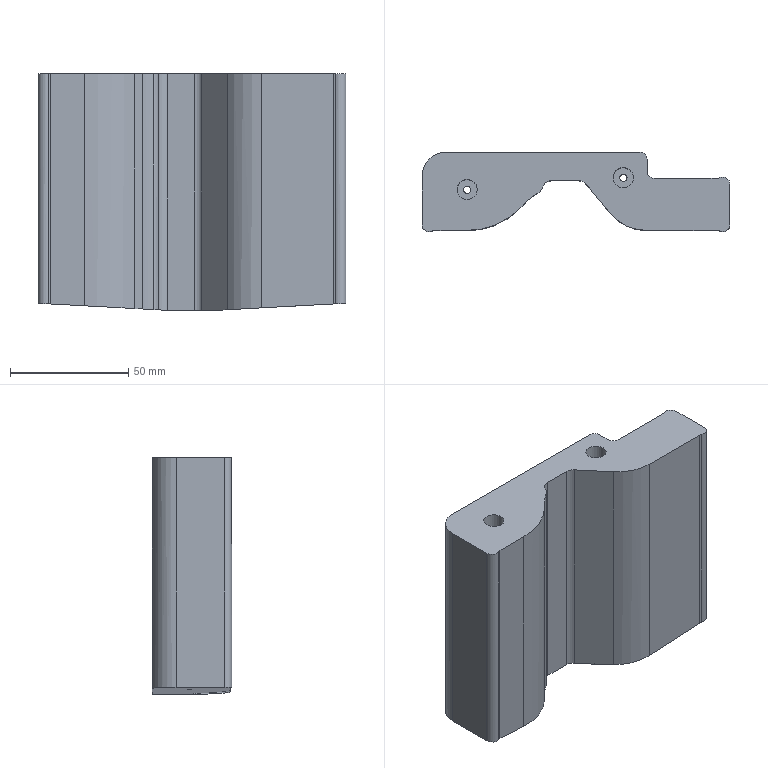Part | STEP file | lll_id242_x_t | 1 solid | 35 faces | box 130 x 33.5 x 100 mm | volume 301852 mm3 | cylinder 19 | plane 16 | commonest cylinder face diameters 6 x8 8 x3 3.1 x2 8.506 x2 20 x1 38 x1
STEP:
#1=CARTESIAN_POINT('',(669.,-7.5,-7.5));
#2=VERTEX_POINT('',#1);
#3=CARTESIAN_POINT('',(669.,-19.5,-7.5));
#4=VERTEX_POINT('',#3);
#5=CARTESIAN_POINT('',(669.,-41.,-7.5));
#6=DIRECTION('',(0.,-1.,0.));
#7=VECTOR('',#6,1.);
#8=LINE('',#5,#7);
#9=EDGE_CURVE('',#2,#4,#8,.T.);
#10=ORIENTED_EDGE('',*,*,#9,.F.);
#11=CARTESIAN_POINT('',(689.,-7.5,-7.5));
#12=VERTEX_POINT('',#11);
#13=CARTESIAN_POINT('',(781.007,-7.5,-7.5));
#14=DIRECTION('',(-1.,0.,0.));
#15=VECTOR('',#14,1.);
#16=LINE('',#13,#15);
#17=EDGE_CURVE('',#12,#2,#16,.T.);
#18=ORIENTED_EDGE('',*,*,#17,.F.);
#19=CARTESIAN_POINT('',(689.,-27.82,-7.5));
#20=VERTEX_POINT('',#19);
#21=CARTESIAN_POINT('',(689.,-41.,-7.5));
#22=DIRECTION('',(0.,1.,0.));
#23=VECTOR('',#22,1.);
#24=LINE('',#21,#23);
#25=EDGE_CURVE('',#20,#12,#24,.T.);
#26=ORIENTED_EDGE('',*,*,#25,.F.);
#27=CARTESIAN_POINT('',(683.218,-20.929,-7.5));
#28=VERTEX_POINT('',#27);
#29=CARTESIAN_POINT('',(689.435,-28.338,-7.5));
#30=DIRECTION('',(0.6428,-0.766,0.));
#31=VECTOR('',#30,1.);
#32=LINE('',#29,#31);
#33=EDGE_CURVE('',#28,#20,#32,.T.);
#34=ORIENTED_EDGE('',*,*,#33,.F.);
#35=CARTESIAN_POINT('',(680.154,-19.5,-7.5));
#36=VERTEX_POINT('',#35);
#37=CARTESIAN_POINT('',(680.154,-23.5,-7.5));
#38=DIRECTION('',(0.,0.,1.));
#39=DIRECTION('',(-1.,0.,0.));
#40=AXIS2_PLACEMENT_3D('',#37,#38,#39);
#41=CIRCLE('',#40,4.);
#42=EDGE_CURVE('',#28,#36,#41,.T.);
#43=ORIENTED_EDGE('',*,*,#42,.T.);
#44=CARTESIAN_POINT('',(781.007,-19.5,-7.5));
#45=DIRECTION('',(-1.,0.,0.));
#46=VECTOR('',#45,1.);
#47=LINE('',#44,#46);
#48=EDGE_CURVE('',#36,#4,#47,.T.);
#49=ORIENTED_EDGE('',*,*,#48,.T.);
#50=EDGE_LOOP('',(#10,#18,#26,#34,#43,#49));
#51=FACE_OUTER_BOUND('',#50,.T.);
#52=CARTESIAN_POINT('',(781.007,48.5,-7.5));
#53=DIRECTION('',(0.,0.,-1.));
#54=DIRECTION('',(1.,0.,0.));
#55=AXIS2_PLACEMENT_3D('',#52,#53,#54);
#56=PLANE('',#55);
#57=ADVANCED_FACE('',(#51),#56,.T.);
#58=CARTESIAN_POINT('',(703.253,-18.25,92.5));
#59=VERTEX_POINT('',#58);
#60=CARTESIAN_POINT('',(699.,-18.25,92.5));
#61=DIRECTION('',(0.,0.,1.));
#62=DIRECTION('',(1.,0.,0.));
#63=AXIS2_PLACEMENT_3D('',#60,#61,#62);
#64=CIRCLE('',#63,4.253);
#65=EDGE_CURVE('',#59,#59,#64,.T.);
#66=ORIENTED_EDGE('',*,*,#65,.F.);
#67=EDGE_LOOP('',(#66));
#68=FACE_BOUND('',#67,.T.);
#69=CARTESIAN_POINT('',(637.253,-23.25,92.5));
#70=VERTEX_POINT('',#69);
#71=CARTESIAN_POINT('',(633.,-23.25,92.5));
#72=DIRECTION('',(0.,0.,1.));
#73=DIRECTION('',(1.,0.,0.));
#74=AXIS2_PLACEMENT_3D('',#71,#72,#73);
#75=CIRCLE('',#74,4.253);
#76=EDGE_CURVE('',#70,#70,#75,.T.);
#77=ORIENTED_EDGE('',*,*,#76,.F.);
#78=EDGE_LOOP('',(#77));
#79=FACE_BOUND('',#78,.T.);
#80=CARTESIAN_POINT('',(708.5,-40.5,92.5));
#81=VERTEX_POINT('',#80);
#82=CARTESIAN_POINT('',(693.945,-33.713,92.5));
#83=VERTEX_POINT('',#82);
#84=CARTESIAN_POINT('',(708.5,-21.5,92.5));
#85=DIRECTION('',(0.,0.,-1.));
#86=DIRECTION('',(1.,0.,0.));
#87=AXIS2_PLACEMENT_3D('',#84,#85,#86);
#88=CIRCLE('',#87,19.);
#89=EDGE_CURVE('',#81,#83,#88,.T.);
#90=ORIENTED_EDGE('',*,*,#89,.F.);
#91=CARTESIAN_POINT('',(738.602,-40.5,92.5));
#92=VERTEX_POINT('',#91);
#93=CARTESIAN_POINT('',(741.,-40.5,92.5));
#94=DIRECTION('',(1.,0.,0.));
#95=VECTOR('',#94,1.);
#96=LINE('',#93,#95);
#97=EDGE_CURVE('',#81,#92,#96,.T.);
#98=ORIENTED_EDGE('',*,*,#97,.T.);
#99=CARTESIAN_POINT('',(739.801,-40.75,92.5));
#100=VERTEX_POINT('',#99);
#101=CARTESIAN_POINT('',(738.602,-43.5,92.5));
#102=DIRECTION('',(0.,0.,-1.));
#103=DIRECTION('',(1.,0.,0.));
#104=AXIS2_PLACEMENT_3D('',#101,#102,#103);
#105=CIRCLE('',#104,3.);
#106=EDGE_CURVE('',#92,#100,#105,.T.);
#107=ORIENTED_EDGE('',*,*,#106,.T.);
#108=CARTESIAN_POINT('',(744.,-38.,92.5));
#109=VERTEX_POINT('',#108);
#110=CARTESIAN_POINT('',(741.,-38.,92.5));
#111=DIRECTION('',(0.,0.,1.));
#112=DIRECTION('',(1.,0.,0.));
#113=AXIS2_PLACEMENT_3D('',#110,#111,#112);
#114=CIRCLE('',#113,3.);
#115=EDGE_CURVE('',#100,#109,#114,.T.);
#116=ORIENTED_EDGE('',*,*,#115,.T.);
#117=CARTESIAN_POINT('',(744.,-21.,92.5));
#118=VERTEX_POINT('',#117);
#119=CARTESIAN_POINT('',(744.,-21.,92.5));
#120=DIRECTION('',(0.,-1.,0.));
#121=VECTOR('',#120,1.);
#122=LINE('',#119,#121);
#123=EDGE_CURVE('',#118,#109,#122,.T.);
#124=ORIENTED_EDGE('',*,*,#123,.F.);
#125=CARTESIAN_POINT('',(739.801,-18.25,92.5));
#126=VERTEX_POINT('',#125);
#127=CARTESIAN_POINT('',(741.,-21.,92.5));
#128=DIRECTION('',(0.,0.,1.));
#129=DIRECTION('',(1.,0.,0.));
#130=AXIS2_PLACEMENT_3D('',#127,#128,#129);
#131=CIRCLE('',#130,3.);
#132=EDGE_CURVE('',#118,#126,#131,.T.);
#133=ORIENTED_EDGE('',*,*,#132,.T.);
#134=CARTESIAN_POINT('',(738.602,-18.5,92.5));
#135=VERTEX_POINT('',#134);
#136=CARTESIAN_POINT('',(738.602,-15.5,92.5));
#137=DIRECTION('',(0.,0.,-1.));
#138=DIRECTION('',(1.,0.,0.));
#139=AXIS2_PLACEMENT_3D('',#136,#137,#138);
#140=CIRCLE('',#139,3.);
#141=EDGE_CURVE('',#126,#135,#140,.T.);
#142=ORIENTED_EDGE('',*,*,#141,.T.);
#143=CARTESIAN_POINT('',(712.,-18.5,92.5));
#144=VERTEX_POINT('',#143);
#145=CARTESIAN_POINT('',(741.,-18.5,92.5));
#146=DIRECTION('',(1.,0.,0.));
#147=VECTOR('',#146,1.);
#148=LINE('',#145,#147);
#149=EDGE_CURVE('',#144,#135,#148,.T.);
#150=ORIENTED_EDGE('',*,*,#149,.F.);
#151=CARTESIAN_POINT('',(709.,-15.5,92.5));
#152=VERTEX_POINT('',#151);
#153=CARTESIAN_POINT('',(712.,-15.5,92.5));
#154=DIRECTION('',(0.,0.,1.));
#155=DIRECTION('',(1.,0.,0.));
#156=AXIS2_PLACEMENT_3D('',#153,#154,#155);
#157=CIRCLE('',#156,3.);
#158=EDGE_CURVE('',#152,#144,#157,.T.);
#159=ORIENTED_EDGE('',*,*,#158,.F.);
#160=CARTESIAN_POINT('',(709.,-10.5,92.5));
#161=VERTEX_POINT('',#160);
#162=CARTESIAN_POINT('',(709.,-21.,92.5));
#163=DIRECTION('',(0.,1.,0.));
#164=VECTOR('',#163,1.);
#165=LINE('',#162,#164);
#166=EDGE_CURVE('',#152,#161,#165,.T.);
#167=ORIENTED_EDGE('',*,*,#166,.T.);
#168=CARTESIAN_POINT('',(706.,-7.5,92.5));
#169=VERTEX_POINT('',#168);
#170=CARTESIAN_POINT('',(706.,-10.5,92.5));
#171=DIRECTION('',(0.,0.,1.));
#172=DIRECTION('',(1.,0.,0.));
#173=AXIS2_PLACEMENT_3D('',#170,#171,#172);
#174=CIRCLE('',#173,3.);
#175=EDGE_CURVE('',#161,#169,#174,.T.);
#176=ORIENTED_EDGE('',*,*,#175,.T.);
#177=CARTESIAN_POINT('',(624.,-7.5,92.5));
#178=VERTEX_POINT('',#177);
#179=CARTESIAN_POINT('',(741.,-7.5,92.5));
#180=DIRECTION('',(1.,0.,0.));
#181=VECTOR('',#180,1.);
#182=LINE('',#179,#181);
#183=EDGE_CURVE('',#178,#169,#182,.T.);
#184=ORIENTED_EDGE('',*,*,#183,.F.);
#185=CARTESIAN_POINT('',(614.,-17.5,92.5));
#186=VERTEX_POINT('',#185);
#187=CARTESIAN_POINT('',(624.,-17.5,92.5));
#188=DIRECTION('',(0.,0.,1.));
#189=DIRECTION('',(1.,0.,0.));
#190=AXIS2_PLACEMENT_3D('',#187,#188,#189);
#191=CIRCLE('',#190,10.);
#192=EDGE_CURVE('',#178,#186,#191,.T.);
#193=ORIENTED_EDGE('',*,*,#192,.T.);
#194=CARTESIAN_POINT('',(614.,-38.,92.5));
#195=VERTEX_POINT('',#194);
#196=CARTESIAN_POINT('',(614.,-21.,92.5));
#197=DIRECTION('',(0.,1.,0.));
#198=VECTOR('',#197,1.);
#199=LINE('',#196,#198);
#200=EDGE_CURVE('',#195,#186,#199,.T.);
#201=ORIENTED_EDGE('',*,*,#200,.F.);
#202=CARTESIAN_POINT('',(618.199,-40.75,92.5));
#203=VERTEX_POINT('',#202);
#204=CARTESIAN_POINT('',(617.,-38.,92.5));
#205=DIRECTION('',(0.,0.,-1.));
#206=DIRECTION('',(1.,0.,0.));
#207=AXIS2_PLACEMENT_3D('',#204,#205,#206);
#208=CIRCLE('',#207,3.);
#209=EDGE_CURVE('',#203,#195,#208,.T.);
#210=ORIENTED_EDGE('',*,*,#209,.F.);
#211=CARTESIAN_POINT('',(619.398,-40.5,92.5));
#212=VERTEX_POINT('',#211);
#213=CARTESIAN_POINT('',(619.398,-43.5,92.5));
#214=DIRECTION('',(0.,0.,1.));
#215=DIRECTION('',(1.,0.,0.));
#216=AXIS2_PLACEMENT_3D('',#213,#214,#215);
#217=CIRCLE('',#216,3.);
#218=EDGE_CURVE('',#212,#203,#217,.T.);
#219=ORIENTED_EDGE('',*,*,#218,.F.);
#220=CARTESIAN_POINT('',(633.574,-40.5,92.5));
#221=VERTEX_POINT('',#220);
#222=CARTESIAN_POINT('',(741.,-40.5,92.5));
#223=DIRECTION('',(1.,0.,0.));
#224=VECTOR('',#223,1.);
#225=LINE('',#222,#224);
#226=EDGE_CURVE('',#212,#221,#225,.T.);
#227=ORIENTED_EDGE('',*,*,#226,.T.);
#228=CARTESIAN_POINT('',(654.787,-31.713,92.5));
#229=VERTEX_POINT('',#228);
#230=CARTESIAN_POINT('',(633.574,-10.502,92.5));
#231=DIRECTION('',(0.,0.,-1.));
#232=DIRECTION('',(1.,0.,0.));
#233=AXIS2_PLACEMENT_3D('',#230,#231,#232);
#234=CIRCLE('',#233,29.998);
#235=EDGE_CURVE('',#229,#221,#234,.T.);
#236=ORIENTED_EDGE('',*,*,#235,.F.);
#237=CARTESIAN_POINT('',(658.142,-28.358,92.5));
#238=VERTEX_POINT('',#237);
#239=CARTESIAN_POINT('',(703.25,16.75,92.5));
#240=DIRECTION('',(0.7071,0.7071,0.));
#241=VECTOR('',#240,1.);
#242=LINE('',#239,#241);
#243=EDGE_CURVE('',#229,#238,#242,.T.);
#244=ORIENTED_EDGE('',*,*,#243,.T.);
#245=CARTESIAN_POINT('',(662.881,-24.849,92.5));
#246=VERTEX_POINT('',#245);
#247=CARTESIAN_POINT('',(672.216,-42.407,92.5));
#248=DIRECTION('',(0.,0.,-1.));
#249=DIRECTION('',(1.,0.,0.));
#250=AXIS2_PLACEMENT_3D('',#247,#248,#249);
#251=CIRCLE('',#250,19.886);
#252=EDGE_CURVE('',#238,#246,#251,.T.);
#253=ORIENTED_EDGE('',*,*,#252,.T.);
#254=CARTESIAN_POINT('',(664.848,-22.409,92.5));
#255=VERTEX_POINT('',#254);
#256=CARTESIAN_POINT('',(661.,-21.318,92.5));
#257=DIRECTION('',(0.,0.,-1.));
#258=DIRECTION('',(1.,0.,0.));
#259=AXIS2_PLACEMENT_3D('',#256,#257,#258);
#260=CIRCLE('',#259,4.);
#261=EDGE_CURVE('',#255,#246,#260,.T.);
#262=ORIENTED_EDGE('',*,*,#261,.F.);
#263=CARTESIAN_POINT('',(668.697,-19.5,92.5));
#264=VERTEX_POINT('',#263);
#265=CARTESIAN_POINT('',(668.697,-23.5,92.5));
#266=DIRECTION('',(0.,0.,1.));
#267=DIRECTION('',(1.,0.,0.));
#268=AXIS2_PLACEMENT_3D('',#265,#266,#267);
#269=CIRCLE('',#268,4.);
#270=EDGE_CURVE('',#264,#255,#269,.T.);
#271=ORIENTED_EDGE('',*,*,#270,.F.);
#272=CARTESIAN_POINT('',(680.154,-19.5,92.5));
#273=VERTEX_POINT('',#272);
#274=CARTESIAN_POINT('',(741.,-19.5,92.5));
#275=DIRECTION('',(-1.,0.,0.));
#276=VECTOR('',#275,1.);
#277=LINE('',#274,#276);
#278=EDGE_CURVE('',#273,#264,#277,.T.);
#279=ORIENTED_EDGE('',*,*,#278,.F.);
#280=CARTESIAN_POINT('',(683.218,-20.929,92.5));
#281=VERTEX_POINT('',#280);
#282=CARTESIAN_POINT('',(680.154,-23.5,92.5));
#283=DIRECTION('',(0.,0.,-1.));
#284=DIRECTION('',(1.,0.,0.));
#285=AXIS2_PLACEMENT_3D('',#282,#283,#284);
#286=CIRCLE('',#285,4.);
#287=EDGE_CURVE('',#273,#281,#286,.T.);
#288=ORIENTED_EDGE('',*,*,#287,.T.);
#289=CARTESIAN_POINT('',(707.127,-49.423,92.5));
#290=DIRECTION('',(-0.6428,0.766,0.));
#291=VECTOR('',#290,1.);
#292=LINE('',#289,#291);
#293=EDGE_CURVE('',#83,#281,#292,.T.);
#294=ORIENTED_EDGE('',*,*,#293,.F.);
#295=EDGE_LOOP('',(#90,#98,#107,#116,#124,#133,#142,#150,#159,#167,#176,#184,#193,#201,#210,#219,#227,#236,#244,#253,#262,#271,#279,#288,#294));
#296=FACE_BOUND('',#295,.T.);
#297=CARTESIAN_POINT('',(741.,-21.,92.5));
#298=DIRECTION('',(0.,0.,1.));
#299=DIRECTION('',(-1.,0.,0.));
#300=AXIS2_PLACEMENT_3D('',#297,#298,#299);
#301=PLANE('',#300);
#302=ADVANCED_FACE('',(#68,#79,#296),#301,.T.);
#303=CARTESIAN_POINT('',(697.45,-18.25,-7.039));
#304=VERTEX_POINT('',#303);
#305=CARTESIAN_POINT('',(699.,-18.25,-6.955));
#306=DIRECTION('',(0.05446,0.,-0.9985));
#307=DIRECTION('',(-0.9985,0.,-0.05446));
#308=AXIS2_PLACEMENT_3D('',#305,#306,#307);
#309=ELLIPSE('',#308,1.552,1.55);
#310=EDGE_CURVE('',#304,#304,#309,.T.);
#311=ORIENTED_EDGE('',*,*,#310,.F.);
#312=EDGE_LOOP('',(#311));
#313=FACE_BOUND('',#312,.T.);
#314=ORIENTED_EDGE('',*,*,#25,.T.);
#315=CARTESIAN_POINT('',(706.,-7.5,-6.573));
#316=VERTEX_POINT('',#315);
#317=CARTESIAN_POINT('',(689.,-7.5,-7.5));
#318=DIRECTION('',(0.9985,0.,0.05446));
#319=VECTOR('',#318,1.);
#320=LINE('',#317,#319);
#321=EDGE_CURVE('',#12,#316,#320,.T.);
#322=ORIENTED_EDGE('',*,*,#321,.T.);
#323=CARTESIAN_POINT('',(709.,-10.5,-6.409));
#324=VERTEX_POINT('',#323);
#325=CARTESIAN_POINT('',(706.,-10.5,-6.573));
#326=DIRECTION('',(0.05446,0.,-0.9985));
#327=DIRECTION('',(0.9985,0.,0.05446));
#328=AXIS2_PLACEMENT_3D('',#325,#326,#327);
#329=ELLIPSE('',#328,3.004,3.);
#330=EDGE_CURVE('',#316,#324,#329,.T.);
#331=ORIENTED_EDGE('',*,*,#330,.T.);
#332=CARTESIAN_POINT('',(709.,-15.5,-6.409));
#333=VERTEX_POINT('',#332);
#334=CARTESIAN_POINT('',(709.,-41.,-6.409));
#335=DIRECTION('',(0.,1.,0.));
#336=VECTOR('',#335,1.);
#337=LINE('',#334,#336);
#338=EDGE_CURVE('',#333,#324,#337,.T.);
#339=ORIENTED_EDGE('',*,*,#338,.F.);
#340=CARTESIAN_POINT('',(712.,-18.5,-6.245));
#341=VERTEX_POINT('',#340);
#342=CARTESIAN_POINT('',(712.,-15.5,-6.245));
#343=DIRECTION('',(-0.05446,0.,0.9985));
#344=DIRECTION('',(0.9985,0.,0.05446));
#345=AXIS2_PLACEMENT_3D('',#342,#343,#344);
#346=ELLIPSE('',#345,3.004,3.);
#347=EDGE_CURVE('',#333,#341,#346,.T.);
#348=ORIENTED_EDGE('',*,*,#347,.T.);
#349=CARTESIAN_POINT('',(738.602,-18.5,-4.794));
#350=VERTEX_POINT('',#349);
#351=CARTESIAN_POINT('',(689.,-18.5,-7.5));
#352=DIRECTION('',(-0.9985,0.,-0.05446));
#353=VECTOR('',#352,1.);
#354=LINE('',#351,#353);
#355=EDGE_CURVE('',#350,#341,#354,.T.);
#356=ORIENTED_EDGE('',*,*,#355,.F.);
#357=CARTESIAN_POINT('',(739.801,-18.25,-4.729));
#358=VERTEX_POINT('',#357);
#359=CARTESIAN_POINT('',(738.602,-15.5,-4.794));
#360=DIRECTION('',(0.05446,0.,-0.9985));
#361=DIRECTION('',(0.9985,0.,0.05446));
#362=AXIS2_PLACEMENT_3D('',#359,#360,#361);
#363=ELLIPSE('',#362,3.004,3.);
#364=EDGE_CURVE('',#358,#350,#363,.T.);
#365=ORIENTED_EDGE('',*,*,#364,.F.);
#366=CARTESIAN_POINT('',(744.,-21.,-4.5));
#367=VERTEX_POINT('',#366);
#368=CARTESIAN_POINT('',(741.,-21.,-4.664));
#369=DIRECTION('',(0.05446,0.,-0.9985));
#370=DIRECTION('',(0.9985,0.,0.05446));
#371=AXIS2_PLACEMENT_3D('',#368,#369,#370);
#372=ELLIPSE('',#371,3.004,3.);
#373=EDGE_CURVE('',#358,#367,#372,.T.);
#374=ORIENTED_EDGE('',*,*,#373,.T.);
#375=CARTESIAN_POINT('',(744.,-38.,-4.5));
#376=VERTEX_POINT('',#375);
#377=CARTESIAN_POINT('',(744.,-41.,-4.5));
#378=DIRECTION('',(0.,-1.,0.));
#379=VECTOR('',#378,1.);
#380=LINE('',#377,#379);
#381=EDGE_CURVE('',#367,#376,#380,.T.);
#382=ORIENTED_EDGE('',*,*,#381,.T.);
#383=CARTESIAN_POINT('',(739.801,-40.75,-4.729));
#384=VERTEX_POINT('',#383);
#385=CARTESIAN_POINT('',(741.,-38.,-4.664));
#386=DIRECTION('',(0.05446,0.,-0.9985));
#387=DIRECTION('',(0.9985,0.,0.05446));
#388=AXIS2_PLACEMENT_3D('',#385,#386,#387);
#389=ELLIPSE('',#388,3.004,3.);
#390=EDGE_CURVE('',#376,#384,#389,.T.);
#391=ORIENTED_EDGE('',*,*,#390,.T.);
#392=CARTESIAN_POINT('',(738.602,-40.5,-4.794));
#393=VERTEX_POINT('',#392);
#394=CARTESIAN_POINT('',(738.602,-43.5,-4.794));
#395=DIRECTION('',(0.05446,0.,-0.9985));
#396=DIRECTION('',(0.9985,0.,0.05446));
#397=AXIS2_PLACEMENT_3D('',#394,#395,#396);
#398=ELLIPSE('',#397,3.004,3.);
#399=EDGE_CURVE('',#393,#384,#398,.T.);
#400=ORIENTED_EDGE('',*,*,#399,.F.);
#401=CARTESIAN_POINT('',(708.5,-40.5,-6.436));
#402=VERTEX_POINT('',#401);
#403=CARTESIAN_POINT('',(689.,-40.5,-7.5));
#404=DIRECTION('',(-0.9985,0.,-0.05446));
#405=VECTOR('',#404,1.);
#406=LINE('',#403,#405);
#407=EDGE_CURVE('',#393,#402,#406,.T.);
#408=ORIENTED_EDGE('',*,*,#407,.T.);
#409=CARTESIAN_POINT('',(693.945,-33.713,-7.23));
#410=VERTEX_POINT('',#409);
#411=CARTESIAN_POINT('',(708.5,-21.5,-6.436));
#412=DIRECTION('',(0.05446,0.,-0.9985));
#413=DIRECTION('',(0.9985,0.,0.05446));
#414=AXIS2_PLACEMENT_3D('',#411,#412,#413);
#415=ELLIPSE('',#414,19.028,19.);
#416=EDGE_CURVE('',#402,#410,#415,.T.);
#417=ORIENTED_EDGE('',*,*,#416,.T.);
#418=CARTESIAN_POINT('',(695.482,-35.545,-7.146));
#419=DIRECTION('',(-0.6424,0.7656,-0.03504));
#420=VECTOR('',#419,1.);
#421=LINE('',#418,#420);
#422=EDGE_CURVE('',#410,#20,#421,.T.);
#423=ORIENTED_EDGE('',*,*,#422,.T.);
#424=EDGE_LOOP('',(#314,#322,#331,#339,#348,#356,#365,#374,#382,#391,#400,#408,#417,#423));
#425=FACE_BOUND('',#424,.T.);
#426=CARTESIAN_POINT('',(689.,-41.,-7.5));
#427=DIRECTION('',(0.05446,0.,-0.9985));
#428=DIRECTION('',(0.9985,0.,0.05446));
#429=AXIS2_PLACEMENT_3D('',#426,#427,#428);
#430=PLANE('',#429);
#431=ADVANCED_FACE('',(#313,#425),#430,.T.);
#432=CARTESIAN_POINT('',(634.55,-23.25,-5.621));
#433=VERTEX_POINT('',#432);
#434=CARTESIAN_POINT('',(633.,-23.25,-5.536));
#435=DIRECTION('',(-0.05446,0.,-0.9985));
#436=DIRECTION('',(0.9985,0.,-0.05446));
#437=AXIS2_PLACEMENT_3D('',#434,#435,#436);
#438=ELLIPSE('',#437,1.552,1.55);
#439=EDGE_CURVE('',#433,#433,#438,.T.);
#440=ORIENTED_EDGE('',*,*,#439,.F.);
#441=EDGE_LOOP('',(#440));
#442=FACE_BOUND('',#441,.T.);
#443=CARTESIAN_POINT('',(624.,-7.5,-5.045));
#444=VERTEX_POINT('',#443);
#445=CARTESIAN_POINT('',(614.,-17.5,-4.5));
#446=VERTEX_POINT('',#445);
#447=CARTESIAN_POINT('',(624.,-17.5,-5.045));
#448=DIRECTION('',(0.05446,0.,0.9985));
#449=DIRECTION('',(-0.9985,0.,0.05446));
#450=AXIS2_PLACEMENT_3D('',#447,#448,#449);
#451=ELLIPSE('',#450,10.015,10.);
#452=EDGE_CURVE('',#444,#446,#451,.T.);
#453=ORIENTED_EDGE('',*,*,#452,.F.);
#454=CARTESIAN_POINT('',(614.,-7.5,-4.5));
#455=DIRECTION('',(-0.9985,0.,0.05446));
#456=VECTOR('',#455,1.);
#457=LINE('',#454,#456);
#458=EDGE_CURVE('',#2,#444,#457,.T.);
#459=ORIENTED_EDGE('',*,*,#458,.F.);
#460=ORIENTED_EDGE('',*,*,#9,.T.);
#461=CARTESIAN_POINT('',(668.697,-19.5,-7.483));
#462=VERTEX_POINT('',#461);
#463=CARTESIAN_POINT('',(614.,-19.5,-4.5));
#464=DIRECTION('',(-0.9985,0.,0.05446));
#465=VECTOR('',#464,1.);
#466=LINE('',#463,#465);
#467=EDGE_CURVE('',#4,#462,#466,.T.);
#468=ORIENTED_EDGE('',*,*,#467,.T.);
#469=CARTESIAN_POINT('',(664.848,-22.409,-7.274));
#470=VERTEX_POINT('',#469);
#471=CARTESIAN_POINT('',(668.697,-23.5,-7.483));
#472=DIRECTION('',(-0.05446,0.,-0.9985));
#473=DIRECTION('',(-0.9985,0.,0.05446));
#474=AXIS2_PLACEMENT_3D('',#471,#472,#473);
#475=ELLIPSE('',#474,4.006,4.);
#476=EDGE_CURVE('',#470,#462,#475,.T.);
#477=ORIENTED_EDGE('',*,*,#476,.F.);
#478=CARTESIAN_POINT('',(662.881,-24.849,-7.166));
#479=VERTEX_POINT('',#478);
#480=CARTESIAN_POINT('',(661.,-21.318,-7.064));
#481=DIRECTION('',(-0.05446,0.,-0.9985));
#482=DIRECTION('',(-0.9985,0.,0.05446));
#483=AXIS2_PLACEMENT_3D('',#480,#481,#482);
#484=ELLIPSE('',#483,4.006,4.);
#485=EDGE_CURVE('',#470,#479,#484,.T.);
#486=ORIENTED_EDGE('',*,*,#485,.T.);
#487=CARTESIAN_POINT('',(658.142,-28.358,-6.908));
#488=VERTEX_POINT('',#487);
#489=CARTESIAN_POINT('',(672.216,-42.407,-7.675));
#490=DIRECTION('',(-0.05446,0.,-0.9985));
#491=DIRECTION('',(-0.9985,0.,0.05446));
#492=AXIS2_PLACEMENT_3D('',#489,#490,#491);
#493=ELLIPSE('',#492,19.915,19.886);
#494=EDGE_CURVE('',#488,#479,#493,.T.);
#495=ORIENTED_EDGE('',*,*,#494,.F.);
#496=CARTESIAN_POINT('',(654.787,-31.713,-6.725));
#497=VERTEX_POINT('',#496);
#498=CARTESIAN_POINT('',(629.727,-56.773,-5.358));
#499=DIRECTION('',(-0.7066,-0.7066,0.03854));
#500=VECTOR('',#499,1.);
#501=LINE('',#498,#500);
#502=EDGE_CURVE('',#488,#497,#501,.T.);
#503=ORIENTED_EDGE('',*,*,#502,.T.);
#504=CARTESIAN_POINT('',(633.574,-40.5,-5.568));
#505=VERTEX_POINT('',#504);
#506=CARTESIAN_POINT('',(633.574,-10.502,-5.568));
#507=DIRECTION('',(-0.05446,0.,-0.9985));
#508=DIRECTION('',(-0.9985,0.,0.05446));
#509=AXIS2_PLACEMENT_3D('',#506,#507,#508);
#510=ELLIPSE('',#509,30.042,29.998);
#511=EDGE_CURVE('',#497,#505,#510,.T.);
#512=ORIENTED_EDGE('',*,*,#511,.T.);
#513=CARTESIAN_POINT('',(619.398,-40.5,-4.794));
#514=VERTEX_POINT('',#513);
#515=CARTESIAN_POINT('',(614.,-40.5,-4.5));
#516=DIRECTION('',(0.9985,0.,-0.05446));
#517=VECTOR('',#516,1.);
#518=LINE('',#515,#517);
#519=EDGE_CURVE('',#514,#505,#518,.T.);
#520=ORIENTED_EDGE('',*,*,#519,.F.);
#521=CARTESIAN_POINT('',(618.199,-40.75,-4.729));
#522=VERTEX_POINT('',#521);
#523=CARTESIAN_POINT('',(619.398,-43.5,-4.794));
#524=DIRECTION('',(-0.05446,0.,-0.9985));
#525=DIRECTION('',(-0.9985,0.,0.05446));
#526=AXIS2_PLACEMENT_3D('',#523,#524,#525);
#527=ELLIPSE('',#526,3.004,3.);
#528=EDGE_CURVE('',#522,#514,#527,.T.);
#529=ORIENTED_EDGE('',*,*,#528,.F.);
#530=CARTESIAN_POINT('',(614.,-38.,-4.5));
#531=VERTEX_POINT('',#530);
#532=CARTESIAN_POINT('',(617.,-38.,-4.664));
#533=DIRECTION('',(0.05446,0.,0.9985));
#534=DIRECTION('',(-0.9985,0.,0.05446));
#535=AXIS2_PLACEMENT_3D('',#532,#533,#534);
#536=ELLIPSE('',#535,3.004,3.);
#537=EDGE_CURVE('',#531,#522,#536,.T.);
#538=ORIENTED_EDGE('',*,*,#537,.F.);
#539=CARTESIAN_POINT('',(614.,-41.,-4.5));
#540=DIRECTION('',(0.,1.,0.));
#541=VECTOR('',#540,1.);
#542=LINE('',#539,#541);
#543=EDGE_CURVE('',#531,#446,#542,.T.);
#544=ORIENTED_EDGE('',*,*,#543,.T.);
#545=EDGE_LOOP('',(#453,#459,#460,#468,#477,#486,#495,#503,#512,#520,#529,#538,#544));
#546=FACE_BOUND('',#545,.T.);
#547=CARTESIAN_POINT('',(614.,-41.,-4.5));
#548=DIRECTION('',(-0.05446,0.,-0.9985));
#549=DIRECTION('',(0.9985,0.,-0.05446));
#550=AXIS2_PLACEMENT_3D('',#547,#548,#549);
#551=PLANE('',#550);
#552=ADVANCED_FACE('',(#442,#546),#551,.T.);
#553=CARTESIAN_POINT('',(631.45,-23.25,30.747));
#554=VERTEX_POINT('',#553);
#555=CARTESIAN_POINT('',(633.,-23.25,30.747));
#556=DIRECTION('',(0.,0.,1.));
#557=DIRECTION('',(-1.,0.,0.));
#558=AXIS2_PLACEMENT_3D('',#555,#556,#557);
#559=CIRCLE('',#558,1.55);
#560=EDGE_CURVE('',#554,#554,#559,.T.);
#561=ORIENTED_EDGE('',*,*,#560,.T.);
#562=EDGE_LOOP('',(#561));
#563=FACE_BOUND('',#562,.T.);
#564=ORIENTED_EDGE('',*,*,#439,.T.);
#565=EDGE_LOOP('',(#564));
#566=FACE_BOUND('',#565,.T.);
#567=CARTESIAN_POINT('',(633.,-23.25,63.747));
#568=DIRECTION('',(0.,0.,-1.));
#569=DIRECTION('',(-1.,0.,0.));
#570=AXIS2_PLACEMENT_3D('',#567,#568,#569);
#571=CYLINDRICAL_SURFACE('',#570,1.55);
#572=ADVANCED_FACE('',(#563,#566),#571,.F.);
#573=CARTESIAN_POINT('',(700.55,-18.25,30.747));
#574=VERTEX_POINT('',#573);
#575=CARTESIAN_POINT('',(699.,-18.25,30.747));
#576=DIRECTION('',(0.,0.,-1.));
#577=DIRECTION('',(1.,0.,0.));
#578=AXIS2_PLACEMENT_3D('',#575,#576,#577);
#579=CIRCLE('',#578,1.55);
#580=EDGE_CURVE('',#574,#574,#579,.T.);
#581=ORIENTED_EDGE('',*,*,#580,.F.);
#582=EDGE_LOOP('',(#581));
#583=FACE_BOUND('',#582,.T.);
#584=ORIENTED_EDGE('',*,*,#310,.T.);
#585=EDGE_LOOP('',(#584));
#586=FACE_BOUND('',#585,.T.);
#587=CARTESIAN_POINT('',(699.,-18.25,63.747));
#588=DIRECTION('',(0.,0.,-1.));
#589=DIRECTION('',(-1.,0.,0.));
#590=AXIS2_PLACEMENT_3D('',#587,#588,#589);
#591=CYLINDRICAL_SURFACE('',#590,1.55);
#592=ADVANCED_FACE('',(#583,#586),#591,.F.);
#593=ORIENTED_EDGE('',*,*,#65,.T.);
#594=EDGE_LOOP('',(#593));
#595=FACE_BOUND('',#594,.T.);
#596=CARTESIAN_POINT('',(694.747,-18.25,30.747));
#597=VERTEX_POINT('',#596);
#598=CARTESIAN_POINT('',(699.,-18.25,30.747));
#599=DIRECTION('',(0.,0.,1.));
#600=DIRECTION('',(-1.,0.,0.));
#601=AXIS2_PLACEMENT_3D('',#598,#599,#600);
#602=CIRCLE('',#601,4.253);
#603=EDGE_CURVE('',#597,#597,#602,.T.);
#604=ORIENTED_EDGE('',*,*,#603,.F.);
#605=EDGE_LOOP('',(#604));
#606=FACE_BOUND('',#605,.T.);
#607=CARTESIAN_POINT('',(699.,-18.25,94.5));
#608=DIRECTION('',(0.,0.,-1.));
#609=DIRECTION('',(1.,0.,0.));
#610=AXIS2_PLACEMENT_3D('',#607,#608,#609);
#611=CYLINDRICAL_SURFACE('',#610,4.253);
#612=ADVANCED_FACE('',(#595,#606),#611,.F.);
#613=ORIENTED_EDGE('',*,*,#76,.T.);
#614=EDGE_LOOP('',(#613));
#615=FACE_BOUND('',#614,.T.);
#616=CARTESIAN_POINT('',(628.747,-23.25,30.747));
#617=VERTEX_POINT('',#616);
#618=CARTESIAN_POINT('',(633.,-23.25,30.747));
#619=DIRECTION('',(0.,0.,-1.));
#620=DIRECTION('',(-1.,0.,0.));
#621=AXIS2_PLACEMENT_3D('',#618,#619,#620);
#622=CIRCLE('',#621,4.253);
#623=EDGE_CURVE('',#617,#617,#622,.T.);
#624=ORIENTED_EDGE('',*,*,#623,.T.);
#625=EDGE_LOOP('',(#624));
#626=FACE_BOUND('',#625,.T.);
#627=CARTESIAN_POINT('',(633.,-23.25,94.5));
#628=DIRECTION('',(0.,0.,-1.));
#629=DIRECTION('',(1.,0.,0.));
#630=AXIS2_PLACEMENT_3D('',#627,#628,#629);
#631=CYLINDRICAL_SURFACE('',#630,4.253);
#632=ADVANCED_FACE('',(#615,#626),#631,.F.);
#633=ORIENTED_EDGE('',*,*,#603,.T.);
#634=EDGE_LOOP('',(#633));
#635=FACE_BOUND('',#634,.T.);
#636=ORIENTED_EDGE('',*,*,#580,.T.);
#637=EDGE_LOOP('',(#636));
#638=FACE_BOUND('',#637,.T.);
#639=CARTESIAN_POINT('',(699.,-18.25,30.747));
#640=DIRECTION('',(0.,0.,1.));
#641=DIRECTION('',(1.,0.,0.));
#642=AXIS2_PLACEMENT_3D('',#639,#640,#641);
#643=PLANE('',#642);
#644=ADVANCED_FACE('',(#635,#638),#643,.T.);
#645=ORIENTED_EDGE('',*,*,#623,.F.);
#646=EDGE_LOOP('',(#645));
#647=FACE_BOUND('',#646,.T.);
#648=ORIENTED_EDGE('',*,*,#560,.F.);
#649=EDGE_LOOP('',(#648));
#650=FACE_BOUND('',#649,.T.);
#651=CARTESIAN_POINT('',(633.,-23.25,30.747));
#652=DIRECTION('',(0.,0.,-1.));
#653=DIRECTION('',(-1.,0.,0.));
#654=AXIS2_PLACEMENT_3D('',#651,#652,#653);
#655=PLANE('',#654);
#656=ADVANCED_FACE('',(#647,#650),#655,.F.);
#657=ORIENTED_EDGE('',*,*,#97,.F.);
#658=CARTESIAN_POINT('',(708.5,-40.5,-177.5));
#659=DIRECTION('',(0.,0.,1.));
#660=VECTOR('',#659,1.);
#661=LINE('',#658,#660);
#662=EDGE_CURVE('',#402,#81,#661,.T.);
#663=ORIENTED_EDGE('',*,*,#662,.F.);
#664=ORIENTED_EDGE('',*,*,#407,.F.);
#665=CARTESIAN_POINT('',(738.602,-40.5,-177.5));
#666=DIRECTION('',(0.,0.,1.));
#667=VECTOR('',#666,1.);
#668=LINE('',#665,#667);
#669=EDGE_CURVE('',#393,#92,#668,.T.);
#670=ORIENTED_EDGE('',*,*,#669,.T.);
#671=EDGE_LOOP('',(#657,#663,#664,#670));
#672=FACE_OUTER_BOUND('',#671,.T.);
#673=CARTESIAN_POINT('',(708.5,-40.5,-177.5));
#674=DIRECTION('',(0.,-1.,0.));
#675=DIRECTION('',(1.,0.,0.));
#676=AXIS2_PLACEMENT_3D('',#673,#674,#675);
#677=PLANE('',#676);
#678=ADVANCED_FACE('',(#672),#677,.T.);
#679=ORIENTED_EDGE('',*,*,#106,.F.);
#680=ORIENTED_EDGE('',*,*,#669,.F.);
#681=ORIENTED_EDGE('',*,*,#399,.T.);
#682=CARTESIAN_POINT('',(739.801,-40.75,-177.5));
#683=DIRECTION('',(0.,0.,1.));
#684=VECTOR('',#683,1.);
#685=LINE('',#682,#684);
#686=EDGE_CURVE('',#384,#100,#685,.T.);
#687=ORIENTED_EDGE('',*,*,#686,.T.);
#688=EDGE_LOOP('',(#679,#680,#681,#687));
#689=FACE_OUTER_BOUND('',#688,.T.);
#690=CARTESIAN_POINT('',(738.602,-43.5,-177.5));
#691=DIRECTION('',(0.,0.,1.));
#692=DIRECTION('',(1.,0.,0.));
#693=AXIS2_PLACEMENT_3D('',#690,#691,#692);
#694=CYLINDRICAL_SURFACE('',#693,3.);
#695=ADVANCED_FACE('',(#689),#694,.F.);
#696=ORIENTED_EDGE('',*,*,#115,.F.);
#697=ORIENTED_EDGE('',*,*,#686,.F.);
#698=ORIENTED_EDGE('',*,*,#390,.F.);
#699=CARTESIAN_POINT('',(744.,-38.,-177.5));
#700=DIRECTION('',(0.,0.,1.));
#701=VECTOR('',#700,1.);
#702=LINE('',#699,#701);
#703=EDGE_CURVE('',#376,#109,#702,.T.);
#704=ORIENTED_EDGE('',*,*,#703,.T.);
#705=EDGE_LOOP('',(#696,#697,#698,#704));
#706=FACE_OUTER_BOUND('',#705,.T.);
#707=CARTESIAN_POINT('',(741.,-38.,-177.5));
#708=DIRECTION('',(0.,0.,1.));
#709=DIRECTION('',(1.,0.,0.));
#710=AXIS2_PLACEMENT_3D('',#707,#708,#709);
#711=CYLINDRICAL_SURFACE('',#710,3.);
#712=ADVANCED_FACE('',(#706),#711,.T.);
#713=ORIENTED_EDGE('',*,*,#123,.T.);
#714=ORIENTED_EDGE('',*,*,#703,.F.);
#715=ORIENTED_EDGE('',*,*,#381,.F.);
#716=CARTESIAN_POINT('',(744.,-21.,-177.5));
#717=DIRECTION('',(0.,0.,1.));
#718=VECTOR('',#717,1.);
#719=LINE('',#716,#718);
#720=EDGE_CURVE('',#367,#118,#719,.T.);
#721=ORIENTED_EDGE('',*,*,#720,.T.);
#722=EDGE_LOOP('',(#713,#714,#715,#721));
#723=FACE_OUTER_BOUND('',#722,.T.);
#724=CARTESIAN_POINT('',(744.,-38.,-177.5));
#725=DIRECTION('',(1.,0.,0.));
#726=DIRECTION('',(0.,1.,0.));
#727=AXIS2_PLACEMENT_3D('',#724,#725,#726);
#728=PLANE('',#727);
#729=ADVANCED_FACE('',(#723),#728,.T.);
#730=ORIENTED_EDGE('',*,*,#132,.F.);
#731=ORIENTED_EDGE('',*,*,#720,.F.);
#732=ORIENTED_EDGE('',*,*,#373,.F.);
#733=CARTESIAN_POINT('',(739.801,-18.25,-177.5));
#734=DIRECTION('',(0.,0.,1.));
#735=VECTOR('',#734,1.);
#736=LINE('',#733,#735);
#737=EDGE_CURVE('',#358,#126,#736,.T.);
#738=ORIENTED_EDGE('',*,*,#737,.T.);
#739=EDGE_LOOP('',(#730,#731,#732,#738));
#740=FACE_OUTER_BOUND('',#739,.T.);
#741=CARTESIAN_POINT('',(741.,-21.,-177.5));
#742=DIRECTION('',(0.,0.,1.));
#743=DIRECTION('',(1.,0.,0.));
#744=AXIS2_PLACEMENT_3D('',#741,#742,#743);
#745=CYLINDRICAL_SURFACE('',#744,3.);
#746=ADVANCED_FACE('',(#740),#745,.T.);
#747=ORIENTED_EDGE('',*,*,#141,.F.);
#748=ORIENTED_EDGE('',*,*,#737,.F.);
#749=ORIENTED_EDGE('',*,*,#364,.T.);
#750=CARTESIAN_POINT('',(738.602,-18.5,-177.5));
#751=DIRECTION('',(0.,0.,1.));
#752=VECTOR('',#751,1.);
#753=LINE('',#750,#752);
#754=EDGE_CURVE('',#350,#135,#753,.T.);
#755=ORIENTED_EDGE('',*,*,#754,.T.);
#756=EDGE_LOOP('',(#747,#748,#749,#755));
#757=FACE_OUTER_BOUND('',#756,.T.);
#758=CARTESIAN_POINT('',(738.602,-15.5,-177.5));
#759=DIRECTION('',(0.,0.,1.));
#760=DIRECTION('',(1.,0.,0.));
#761=AXIS2_PLACEMENT_3D('',#758,#759,#760);
#762=CYLINDRICAL_SURFACE('',#761,3.);
#763=ADVANCED_FACE('',(#757),#762,.F.);
#764=ORIENTED_EDGE('',*,*,#149,.T.);
#765=ORIENTED_EDGE('',*,*,#754,.F.);
#766=ORIENTED_EDGE('',*,*,#355,.T.);
#767=CARTESIAN_POINT('',(712.,-18.5,-177.5));
#768=DIRECTION('',(0.,0.,1.));
#769=VECTOR('',#768,1.);
#770=LINE('',#767,#769);
#771=EDGE_CURVE('',#341,#144,#770,.T.);
#772=ORIENTED_EDGE('',*,*,#771,.T.);
#773=EDGE_LOOP('',(#764,#765,#766,#772));
#774=FACE_OUTER_BOUND('',#773,.T.);
#775=CARTESIAN_POINT('',(738.602,-18.5,-177.5));
#776=DIRECTION('',(0.,1.,0.));
#777=DIRECTION('',(-1.,0.,0.));
#778=AXIS2_PLACEMENT_3D('',#775,#776,#777);
#779=PLANE('',#778);
#780=ADVANCED_FACE('',(#774),#779,.T.);
#781=ORIENTED_EDGE('',*,*,#158,.T.);
#782=ORIENTED_EDGE('',*,*,#771,.F.);
#783=ORIENTED_EDGE('',*,*,#347,.F.);
#784=CARTESIAN_POINT('',(709.,-15.5,-177.5));
#785=DIRECTION('',(0.,0.,1.));
#786=VECTOR('',#785,1.);
#787=LINE('',#784,#786);
#788=EDGE_CURVE('',#333,#152,#787,.T.);
#789=ORIENTED_EDGE('',*,*,#788,.T.);
#790=EDGE_LOOP('',(#781,#782,#783,#789));
#791=FACE_OUTER_BOUND('',#790,.T.);
#792=CARTESIAN_POINT('',(712.,-15.5,-177.5));
#793=DIRECTION('',(0.,0.,1.));
#794=DIRECTION('',(1.,0.,0.));
#795=AXIS2_PLACEMENT_3D('',#792,#793,#794);
#796=CYLINDRICAL_SURFACE('',#795,3.);
#797=ADVANCED_FACE('',(#791),#796,.F.);
#798=ORIENTED_EDGE('',*,*,#166,.F.);
#799=ORIENTED_EDGE('',*,*,#788,.F.);
#800=ORIENTED_EDGE('',*,*,#338,.T.);
#801=CARTESIAN_POINT('',(709.,-10.5,-177.5));
#802=DIRECTION('',(0.,0.,1.));
#803=VECTOR('',#802,1.);
#804=LINE('',#801,#803);
#805=EDGE_CURVE('',#324,#161,#804,.T.);
#806=ORIENTED_EDGE('',*,*,#805,.T.);
#807=EDGE_LOOP('',(#798,#799,#800,#806));
#808=FACE_OUTER_BOUND('',#807,.T.);
#809=CARTESIAN_POINT('',(709.,-15.5,-177.5));
#810=DIRECTION('',(1.,0.,0.));
#811=DIRECTION('',(0.,1.,0.));
#812=AXIS2_PLACEMENT_3D('',#809,#810,#811);
#813=PLANE('',#812);
#814=ADVANCED_FACE('',(#808),#813,.T.);
#815=ORIENTED_EDGE('',*,*,#175,.F.);
#816=ORIENTED_EDGE('',*,*,#805,.F.);
#817=ORIENTED_EDGE('',*,*,#330,.F.);
#818=CARTESIAN_POINT('',(706.,-7.5,-177.5));
#819=DIRECTION('',(0.,0.,1.));
#820=VECTOR('',#819,1.);
#821=LINE('',#818,#820);
#822=EDGE_CURVE('',#316,#169,#821,.T.);
#823=ORIENTED_EDGE('',*,*,#822,.T.);
#824=EDGE_LOOP('',(#815,#816,#817,#823));
#825=FACE_OUTER_BOUND('',#824,.T.);
#826=CARTESIAN_POINT('',(706.,-10.5,-177.5));
#827=DIRECTION('',(0.,0.,1.));
#828=DIRECTION('',(1.,0.,0.));
#829=AXIS2_PLACEMENT_3D('',#826,#827,#828);
#830=CYLINDRICAL_SURFACE('',#829,3.);
#831=ADVANCED_FACE('',(#825),#830,.T.);
#832=ORIENTED_EDGE('',*,*,#183,.T.);
#833=ORIENTED_EDGE('',*,*,#822,.F.);
#834=ORIENTED_EDGE('',*,*,#321,.F.);
#835=ORIENTED_EDGE('',*,*,#17,.T.);
#836=ORIENTED_EDGE('',*,*,#458,.T.);
#837=CARTESIAN_POINT('',(624.,-7.5,-177.5));
#838=DIRECTION('',(0.,0.,1.));
#839=VECTOR('',#838,1.);
#840=LINE('',#837,#839);
#841=EDGE_CURVE('',#444,#178,#840,.T.);
#842=ORIENTED_EDGE('',*,*,#841,.T.);
#843=EDGE_LOOP('',(#832,#833,#834,#835,#836,#842));
#844=FACE_OUTER_BOUND('',#843,.T.);
#845=CARTESIAN_POINT('',(706.,-7.5,-177.5));
#846=DIRECTION('',(0.,1.,0.));
#847=DIRECTION('',(-1.,0.,0.));
#848=AXIS2_PLACEMENT_3D('',#845,#846,#847);
#849=PLANE('',#848);
#850=ADVANCED_FACE('',(#844),#849,.T.);
#851=ORIENTED_EDGE('',*,*,#192,.F.);
#852=ORIENTED_EDGE('',*,*,#841,.F.);
#853=ORIENTED_EDGE('',*,*,#452,.T.);
#854=CARTESIAN_POINT('',(614.,-17.5,-177.5));
#855=DIRECTION('',(0.,0.,1.));
#856=VECTOR('',#855,1.);
#857=LINE('',#854,#856);
#858=EDGE_CURVE('',#446,#186,#857,.T.);
#859=ORIENTED_EDGE('',*,*,#858,.T.);
#860=EDGE_LOOP('',(#851,#852,#853,#859));
#861=FACE_OUTER_BOUND('',#860,.T.);
#862=CARTESIAN_POINT('',(624.,-17.5,-177.5));
#863=DIRECTION('',(0.,0.,1.));
#864=DIRECTION('',(1.,0.,0.));
#865=AXIS2_PLACEMENT_3D('',#862,#863,#864);
#866=CYLINDRICAL_SURFACE('',#865,10.);
#867=ADVANCED_FACE('',(#861),#866,.T.);
#868=ORIENTED_EDGE('',*,*,#200,.T.);
#869=ORIENTED_EDGE('',*,*,#858,.F.);
#870=ORIENTED_EDGE('',*,*,#543,.F.);
#871=CARTESIAN_POINT('',(614.,-38.,-177.5));
#872=DIRECTION('',(0.,0.,1.));
#873=VECTOR('',#872,1.);
#874=LINE('',#871,#873);
#875=EDGE_CURVE('',#531,#195,#874,.T.);
#876=ORIENTED_EDGE('',*,*,#875,.T.);
#877=EDGE_LOOP('',(#868,#869,#870,#876));
#878=FACE_OUTER_BOUND('',#877,.T.);
#879=CARTESIAN_POINT('',(614.,-17.5,-177.5));
#880=DIRECTION('',(-1.,0.,0.));
#881=DIRECTION('',(0.,0.,1.));
#882=AXIS2_PLACEMENT_3D('',#879,#880,#881);
#883=PLANE('',#882);
#884=ADVANCED_FACE('',(#878),#883,.T.);
#885=ORIENTED_EDGE('',*,*,#209,.T.);
#886=ORIENTED_EDGE('',*,*,#875,.F.);
#887=ORIENTED_EDGE('',*,*,#537,.T.);
#888=CARTESIAN_POINT('',(618.199,-40.75,-177.5));
#889=DIRECTION('',(0.,0.,1.));
#890=VECTOR('',#889,1.);
#891=LINE('',#888,#890);
#892=EDGE_CURVE('',#522,#203,#891,.T.);
#893=ORIENTED_EDGE('',*,*,#892,.T.);
#894=EDGE_LOOP('',(#885,#886,#887,#893));
#895=FACE_OUTER_BOUND('',#894,.T.);
#896=CARTESIAN_POINT('',(617.,-38.,-177.5));
#897=DIRECTION('',(0.,0.,1.));
#898=DIRECTION('',(1.,0.,0.));
#899=AXIS2_PLACEMENT_3D('',#896,#897,#898);
#900=CYLINDRICAL_SURFACE('',#899,3.);
#901=ADVANCED_FACE('',(#895),#900,.T.);
#902=ORIENTED_EDGE('',*,*,#218,.T.);
#903=ORIENTED_EDGE('',*,*,#892,.F.);
#904=ORIENTED_EDGE('',*,*,#528,.T.);
#905=CARTESIAN_POINT('',(619.398,-40.5,-177.5));
#906=DIRECTION('',(0.,0.,1.));
#907=VECTOR('',#906,1.);
#908=LINE('',#905,#907);
#909=EDGE_CURVE('',#514,#212,#908,.T.);
#910=ORIENTED_EDGE('',*,*,#909,.T.);
#911=EDGE_LOOP('',(#902,#903,#904,#910));
#912=FACE_OUTER_BOUND('',#911,.T.);
#913=CARTESIAN_POINT('',(619.398,-43.5,-177.5));
#914=DIRECTION('',(0.,0.,1.));
#915=DIRECTION('',(1.,0.,0.));
#916=AXIS2_PLACEMENT_3D('',#913,#914,#915);
#917=CYLINDRICAL_SURFACE('',#916,3.);
#918=ADVANCED_FACE('',(#912),#917,.F.);
#919=ORIENTED_EDGE('',*,*,#226,.F.);
#920=ORIENTED_EDGE('',*,*,#909,.F.);
#921=ORIENTED_EDGE('',*,*,#519,.T.);
#922=CARTESIAN_POINT('',(633.574,-40.5,-177.5));
#923=DIRECTION('',(0.,0.,1.));
#924=VECTOR('',#923,1.);
#925=LINE('',#922,#924);
#926=EDGE_CURVE('',#505,#221,#925,.T.);
#927=ORIENTED_EDGE('',*,*,#926,.T.);
#928=EDGE_LOOP('',(#919,#920,#921,#927));
#929=FACE_OUTER_BOUND('',#928,.T.);
#930=CARTESIAN_POINT('',(619.398,-40.5,-177.5));
#931=DIRECTION('',(0.,-1.,0.));
#932=DIRECTION('',(1.,0.,0.));
#933=AXIS2_PLACEMENT_3D('',#930,#931,#932);
#934=PLANE('',#933);
#935=ADVANCED_FACE('',(#929),#934,.T.);
#936=ORIENTED_EDGE('',*,*,#235,.T.);
#937=ORIENTED_EDGE('',*,*,#926,.F.);
#938=ORIENTED_EDGE('',*,*,#511,.F.);
#939=CARTESIAN_POINT('',(654.787,-31.713,-177.5));
#940=DIRECTION('',(0.,0.,1.));
#941=VECTOR('',#940,1.);
#942=LINE('',#939,#941);
#943=EDGE_CURVE('',#497,#229,#942,.T.);
#944=ORIENTED_EDGE('',*,*,#943,.T.);
#945=EDGE_LOOP('',(#936,#937,#938,#944));
#946=FACE_OUTER_BOUND('',#945,.T.);
#947=CARTESIAN_POINT('',(633.574,-10.502,-177.5));
#948=DIRECTION('',(0.,0.,1.));
#949=DIRECTION('',(1.,0.,0.));
#950=AXIS2_PLACEMENT_3D('',#947,#948,#949);
#951=CYLINDRICAL_SURFACE('',#950,29.998);
#952=ADVANCED_FACE('',(#946),#951,.T.);
#953=ORIENTED_EDGE('',*,*,#243,.F.);
#954=ORIENTED_EDGE('',*,*,#943,.F.);
#955=ORIENTED_EDGE('',*,*,#502,.F.);
#956=CARTESIAN_POINT('',(658.142,-28.358,-177.5));
#957=DIRECTION('',(0.,0.,1.));
#958=VECTOR('',#957,1.);
#959=LINE('',#956,#958);
#960=EDGE_CURVE('',#488,#238,#959,.T.);
#961=ORIENTED_EDGE('',*,*,#960,.T.);
#962=EDGE_LOOP('',(#953,#954,#955,#961));
#963=FACE_OUTER_BOUND('',#962,.T.);
#964=CARTESIAN_POINT('',(654.787,-31.713,-177.5));
#965=DIRECTION('',(0.7071,-0.7071,0.));
#966=DIRECTION('',(0.7071,0.7071,0.));
#967=AXIS2_PLACEMENT_3D('',#964,#965,#966);
#968=PLANE('',#967);
#969=ADVANCED_FACE('',(#963),#968,.T.);
#970=ORIENTED_EDGE('',*,*,#252,.F.);
#971=ORIENTED_EDGE('',*,*,#960,.F.);
#972=ORIENTED_EDGE('',*,*,#494,.T.);
#973=CARTESIAN_POINT('',(662.881,-24.849,-177.5));
#974=DIRECTION('',(0.,0.,1.));
#975=VECTOR('',#974,1.);
#976=LINE('',#973,#975);
#977=EDGE_CURVE('',#479,#246,#976,.T.);
#978=ORIENTED_EDGE('',*,*,#977,.T.);
#979=EDGE_LOOP('',(#970,#971,#972,#978));
#980=FACE_OUTER_BOUND('',#979,.T.);
#981=CARTESIAN_POINT('',(672.216,-42.407,-177.5));
#982=DIRECTION('',(0.,0.,1.));
#983=DIRECTION('',(1.,0.,0.));
#984=AXIS2_PLACEMENT_3D('',#981,#982,#983);
#985=CYLINDRICAL_SURFACE('',#984,19.886);
#986=ADVANCED_FACE('',(#980),#985,.F.);
#987=ORIENTED_EDGE('',*,*,#261,.T.);
#988=ORIENTED_EDGE('',*,*,#977,.F.);
#989=ORIENTED_EDGE('',*,*,#485,.F.);
#990=CARTESIAN_POINT('',(664.848,-22.409,-177.5));
#991=DIRECTION('',(0.,0.,1.));
#992=VECTOR('',#991,1.);
#993=LINE('',#990,#992);
#994=EDGE_CURVE('',#470,#255,#993,.T.);
#995=ORIENTED_EDGE('',*,*,#994,.T.);
#996=EDGE_LOOP('',(#987,#988,#989,#995));
#997=FACE_OUTER_BOUND('',#996,.T.);
#998=CARTESIAN_POINT('',(661.,-21.318,-177.5));
#999=DIRECTION('',(0.,0.,1.));
#1000=DIRECTION('',(1.,0.,0.));
#1001=AXIS2_PLACEMENT_3D('',#998,#999,#1000);
#1002=CYLINDRICAL_SURFACE('',#1001,4.);
#1003=ADVANCED_FACE('',(#997),#1002,.T.);
#1004=ORIENTED_EDGE('',*,*,#270,.T.);
#1005=ORIENTED_EDGE('',*,*,#994,.F.);
#1006=ORIENTED_EDGE('',*,*,#476,.T.);
#1007=CARTESIAN_POINT('',(668.697,-19.5,-177.5));
#1008=DIRECTION('',(0.,0.,1.));
#1009=VECTOR('',#1008,1.);
#1010=LINE('',#1007,#1009);
#1011=EDGE_CURVE('',#462,#264,#1010,.T.);
#1012=ORIENTED_EDGE('',*,*,#1011,.T.);
#1013=EDGE_LOOP('',(#1004,#1005,#1006,#1012));
#1014=FACE_OUTER_BOUND('',#1013,.T.);
#1015=CARTESIAN_POINT('',(668.697,-23.5,-177.5));
#1016=DIRECTION('',(0.,0.,1.));
#1017=DIRECTION('',(1.,0.,0.));
#1018=AXIS2_PLACEMENT_3D('',#1015,#1016,#1017);
#1019=CYLINDRICAL_SURFACE('',#1018,4.);
#1020=ADVANCED_FACE('',(#1014),#1019,.F.);
#1021=ORIENTED_EDGE('',*,*,#278,.T.);
#1022=ORIENTED_EDGE('',*,*,#1011,.F.);
#1023=ORIENTED_EDGE('',*,*,#467,.F.);
#1024=ORIENTED_EDGE('',*,*,#48,.F.);
#1025=CARTESIAN_POINT('',(680.154,-19.5,-177.5));
#1026=DIRECTION('',(0.,0.,1.));
#1027=VECTOR('',#1026,1.);
#1028=LINE('',#1025,#1027);
#1029=EDGE_CURVE('',#36,#273,#1028,.T.);
#1030=ORIENTED_EDGE('',*,*,#1029,.T.);
#1031=EDGE_LOOP('',(#1021,#1022,#1023,#1024,#1030));
#1032=FACE_OUTER_BOUND('',#1031,.T.);
#1033=CARTESIAN_POINT('',(668.697,-19.5,-177.5));
#1034=DIRECTION('',(0.,-1.,0.));
#1035=DIRECTION('',(1.,0.,0.));
#1036=AXIS2_PLACEMENT_3D('',#1033,#1034,#1035);
#1037=PLANE('',#1036);
#1038=ADVANCED_FACE('',(#1032),#1037,.T.);
#1039=ORIENTED_EDGE('',*,*,#42,.F.);
#1040=CARTESIAN_POINT('',(683.218,-20.929,-177.5));
#1041=DIRECTION('',(0.,0.,1.));
#1042=VECTOR('',#1041,1.);
#1043=LINE('',#1040,#1042);
#1044=EDGE_CURVE('',#28,#281,#1043,.T.);
#1045=ORIENTED_EDGE('',*,*,#1044,.T.);
#1046=ORIENTED_EDGE('',*,*,#287,.F.);
#1047=ORIENTED_EDGE('',*,*,#1029,.F.);
#1048=EDGE_LOOP('',(#1039,#1045,#1046,#1047));
#1049=FACE_OUTER_BOUND('',#1048,.T.);
#1050=CARTESIAN_POINT('',(680.154,-23.5,-177.5));
#1051=DIRECTION('',(0.,0.,1.));
#1052=DIRECTION('',(1.,0.,0.));
#1053=AXIS2_PLACEMENT_3D('',#1050,#1051,#1052);
#1054=CYLINDRICAL_SURFACE('',#1053,4.);
#1055=ADVANCED_FACE('',(#1049),#1054,.F.);
#1056=ORIENTED_EDGE('',*,*,#293,.T.);
#1057=ORIENTED_EDGE('',*,*,#1044,.F.);
#1058=ORIENTED_EDGE('',*,*,#33,.T.);
#1059=ORIENTED_EDGE('',*,*,#422,.F.);
#1060=CARTESIAN_POINT('',(693.945,-33.713,-177.5));
#1061=DIRECTION('',(0.,0.,1.));
#1062=VECTOR('',#1061,1.);
#1063=LINE('',#1060,#1062);
#1064=EDGE_CURVE('',#410,#83,#1063,.T.);
#1065=ORIENTED_EDGE('',*,*,#1064,.T.);
#1066=EDGE_LOOP('',(#1056,#1057,#1058,#1059,#1065));
#1067=FACE_OUTER_BOUND('',#1066,.T.);
#1068=CARTESIAN_POINT('',(683.218,-20.929,-177.5));
#1069=DIRECTION('',(-0.766,-0.6428,0.));
#1070=DIRECTION('',(0.6428,-0.766,0.));
#1071=AXIS2_PLACEMENT_3D('',#1068,#1069,#1070);
#1072=PLANE('',#1071);
#1073=ADVANCED_FACE('',(#1067),#1072,.T.);
#1074=ORIENTED_EDGE('',*,*,#89,.T.);
#1075=ORIENTED_EDGE('',*,*,#1064,.F.);
#1076=ORIENTED_EDGE('',*,*,#416,.F.);
#1077=ORIENTED_EDGE('',*,*,#662,.T.);
#1078=EDGE_LOOP('',(#1074,#1075,#1076,#1077));
#1079=FACE_OUTER_BOUND('',#1078,.T.);
#1080=CARTESIAN_POINT('',(708.5,-21.5,-177.5));
#1081=DIRECTION('',(0.,0.,1.));
#1082=DIRECTION('',(1.,0.,0.));
#1083=AXIS2_PLACEMENT_3D('',#1080,#1081,#1082);
#1084=CYLINDRICAL_SURFACE('',#1083,19.);
#1085=ADVANCED_FACE('',(#1079),#1084,.T.);
#1086=CLOSED_SHELL('',(#57,#302,#431,#552,#572,#592,#612,#632,#644,#656,#678,#695,#712,#729,#746,#763,#780,#797,#814,#831,#850,#867,#884,#901,#918,#935,#952,#969,#986,#1003,#1020,#1038,#1055,#1073,#1085));
#1087=MANIFOLD_SOLID_BREP('',#1086);
#1088=(LENGTH_UNIT()NAMED_UNIT(*)SI_UNIT(.MILLI.,.METRE.));
#1089=UNCERTAINTY_MEASURE_WITH_UNIT(LENGTH_MEASURE(0.00002),#1088,'','');
#1090=(NAMED_UNIT(*)PLANE_ANGLE_UNIT()SI_UNIT($,.RADIAN.));
#1091=PLANE_ANGLE_MEASURE_WITH_UNIT(PLANE_ANGLE_MEASURE(0.01745),#1090);
#1092=DIMENSIONAL_EXPONENTS(0.,0.,0.,0.,0.,0.,0.);
#1093=(CONVERSION_BASED_UNIT('DEGREE',#1091)NAMED_UNIT(#1092)PLANE_ANGLE_UNIT());
#1094=(NAMED_UNIT(*)SI_UNIT($,.STERADIAN.)SOLID_ANGLE_UNIT());
#1095=(GEOMETRIC_REPRESENTATION_CONTEXT(3)GLOBAL_UNCERTAINTY_ASSIGNED_CONTEXT((#1089))GLOBAL_UNIT_ASSIGNED_CONTEXT((#1088,#1093,#1094))REPRESENTATION_CONTEXT('',''));
#1096=ADVANCED_BREP_SHAPE_REPRESENTATION('',(#1087),#1095);